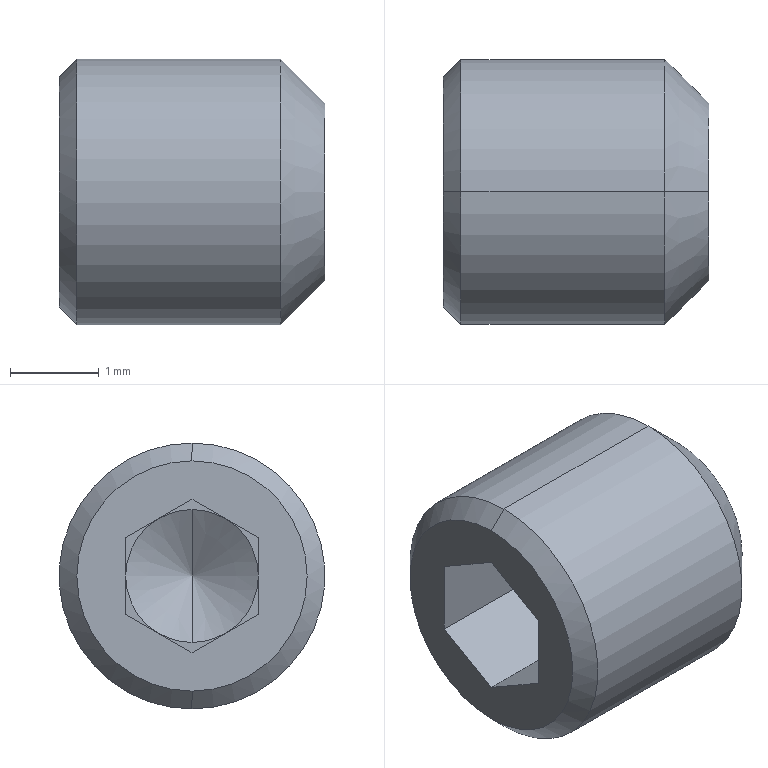Part | SolidWorks | features RevCut 2, Cut 1, LPattern 1, Revolution 1 | 1 solid | 22 faces | box 3 x 3 x 3 mm | volume 17.39 mm3 | plane 14 | cone 6 | cylinder 2 | commonest cylinder face diameters 3 x2